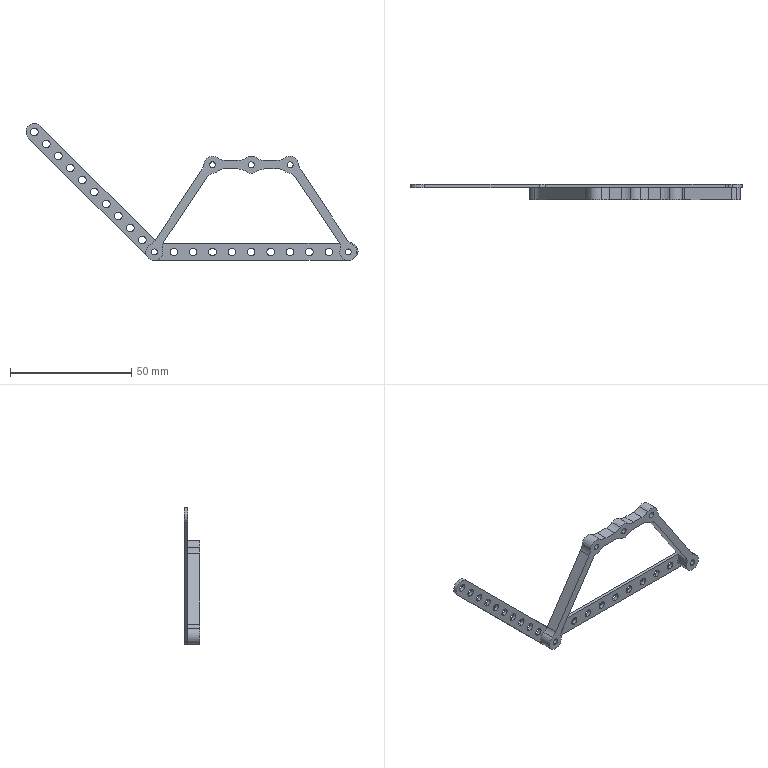Part | SolidWorks | features Fillet 5, ICE 3, Extrusion 1 | 2 solids | 104 faces | box 137.074 x 6.5 x 56.497 mm | volume 3888 mm3 | cylinder 87 | plane 17 | commonest cylinder face diameters 3.1 x42 7 x16 2.5 x10 12 x10 6 x6 8.153 x2